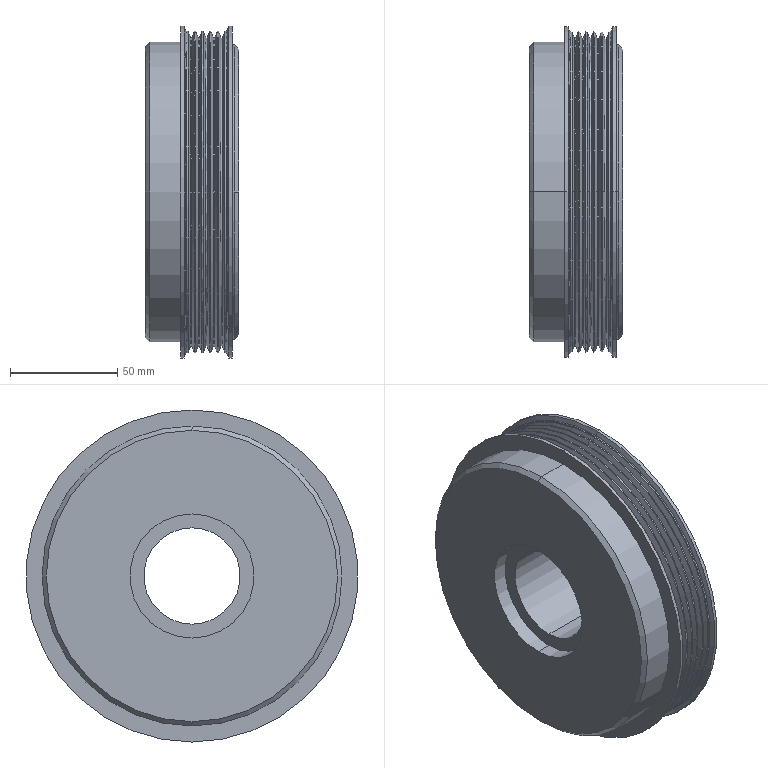Part | STEP file | PN_0001 rotor | 1 solid | 77 faces | box 43.5 x 155 x 155 mm | volume 349048 mm3 | cylinder 38 | cone 28 | plane 7 | spline 4 | commonest cylinder face diameters 150 x12 143.8 x10 155 x4 45 x2 58 x2 85 x2